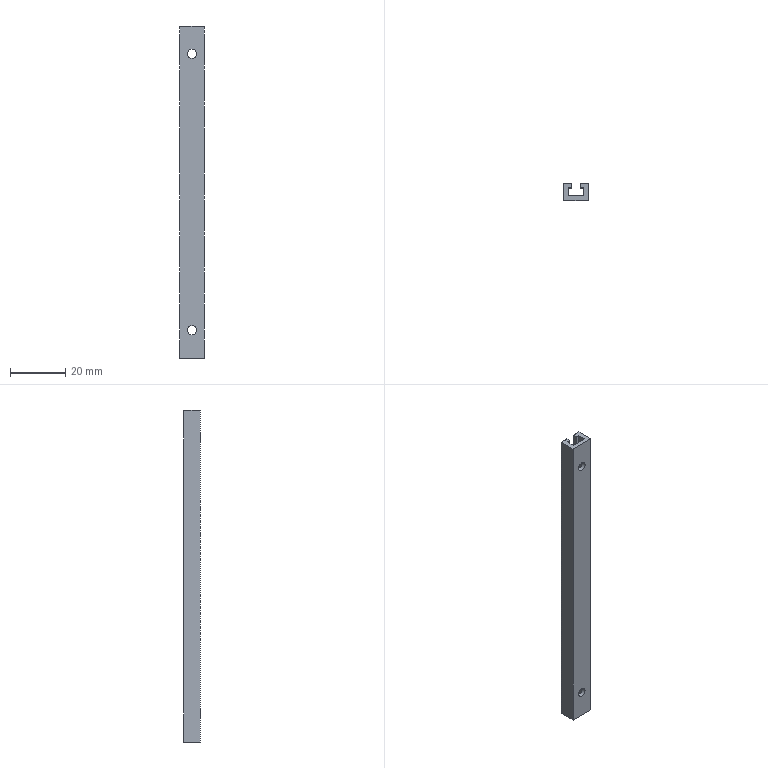Part | NX | 1 solid | 1385 faces | box 9 x 6 x 120 mm | volume 3755 mm3 | plane 1159 | spline 220 | cylinder 6 | commonest cylinder face diameters 6 x4 3.3 x2